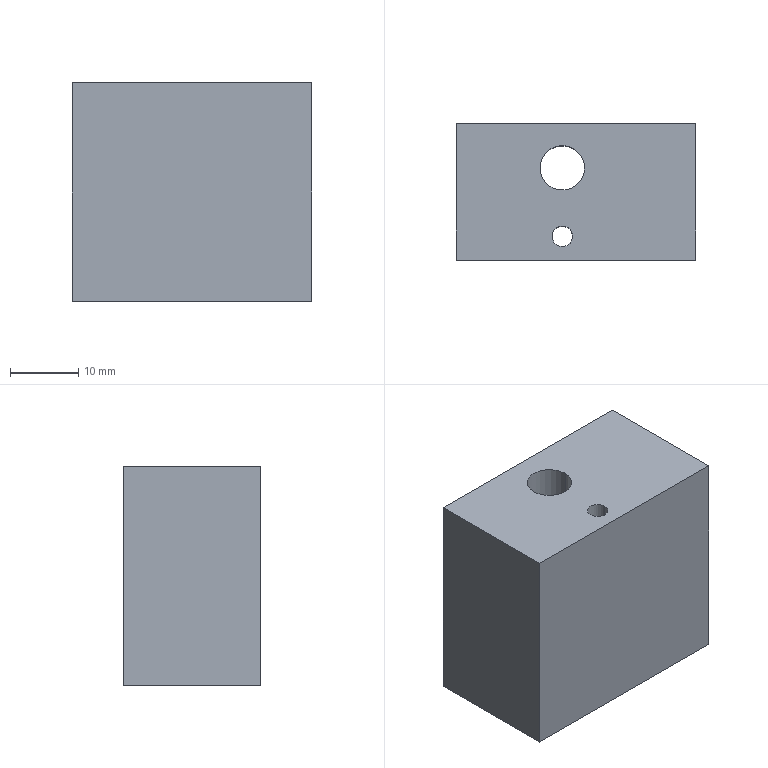Part | SolidWorks | features Cut 2, Extrusion 1, HoleWzd 1 | 1 solid | 18 faces | box 35 x 20 x 32 mm | volume 21036 mm3 | cylinder 8 | plane 6 | cone 4 | commonest cylinder face diameters 2.5 x4 3 x2 6.5 x2
STEP:
#1=CARTESIAN_POINT('',(-8.,12.5,-2.25));
#2=VERTEX_POINT('',#1);
#3=CARTESIAN_POINT('',(-8.,12.5,0.25));
#4=VERTEX_POINT('',#3);
#5=CARTESIAN_POINT('',(-8.,12.5,-1.));
#6=DIRECTION('',(0.,1.,0.));
#7=DIRECTION('',(0.,0.,1.));
#8=AXIS2_PLACEMENT_3D('',#5,#6,#7);
#9=CIRCLE('',#8,1.25);
#10=EDGE_CURVE('',#2,#4,#9,.T.);
#11=ORIENTED_EDGE('',*,*,#10,.F.);
#12=CARTESIAN_POINT('',(-8.,20.,-2.25));
#13=VERTEX_POINT('',#12);
#14=CARTESIAN_POINT('',(-8.,20.,-2.25));
#15=DIRECTION('',(0.,1.,0.));
#16=VECTOR('',#15,1000.);
#17=LINE('',#14,#16);
#18=EDGE_CURVE('',#2,#13,#17,.T.);
#19=ORIENTED_EDGE('',*,*,#18,.T.);
#20=CARTESIAN_POINT('',(-8.,20.,0.25));
#21=VERTEX_POINT('',#20);
#22=CARTESIAN_POINT('',(-8.,20.,-1.));
#23=DIRECTION('',(0.,1.,0.));
#24=DIRECTION('',(0.,0.,1.));
#25=AXIS2_PLACEMENT_3D('',#22,#23,#24);
#26=CIRCLE('',#25,1.25);
#27=EDGE_CURVE('',#13,#21,#26,.T.);
#28=ORIENTED_EDGE('',*,*,#27,.T.);
#29=CARTESIAN_POINT('',(-8.,20.,0.25));
#30=DIRECTION('',(0.,1.,0.));
#31=VECTOR('',#30,1000.);
#32=LINE('',#29,#31);
#33=EDGE_CURVE('',#4,#21,#32,.T.);
#34=ORIENTED_EDGE('',*,*,#33,.F.);
#35=EDGE_LOOP('',(#11,#19,#28,#34));
#36=FACE_OUTER_BOUND('',#35,.T.);
#37=CARTESIAN_POINT('',(-8.,20.,-1.));
#38=DIRECTION('',(0.,1.,0.));
#39=DIRECTION('',(0.,0.,1.));
#40=AXIS2_PLACEMENT_3D('',#37,#38,#39);
#41=CYLINDRICAL_SURFACE('',#40,1.25);
#42=ADVANCED_FACE('',(#36),#41,.F.);
#43=CARTESIAN_POINT('',(-8.,11.749,-1.));
#44=VERTEX_POINT('',#43);
#45=CARTESIAN_POINT('',(-8.,12.5,0.25));
#46=DIRECTION('',(0.,0.515,0.8572));
#47=VECTOR('',#46,1000.);
#48=LINE('',#45,#47);
#49=EDGE_CURVE('',#44,#4,#48,.T.);
#50=ORIENTED_EDGE('',*,*,#49,.F.);
#51=CARTESIAN_POINT('',(-8.,12.5,-2.25));
#52=DIRECTION('',(0.,0.515,-0.8572));
#53=VECTOR('',#52,1000.);
#54=LINE('',#51,#53);
#55=EDGE_CURVE('',#44,#2,#54,.T.);
#56=ORIENTED_EDGE('',*,*,#55,.T.);
#57=ORIENTED_EDGE('',*,*,#10,.T.);
#58=EDGE_LOOP('',(#50,#56,#57));
#59=FACE_OUTER_BOUND('',#58,.T.);
#60=CARTESIAN_POINT('',(-8.,12.5,-1.));
#61=DIRECTION('',(0.,1.,0.));
#62=DIRECTION('',(0.,0.,1.));
#63=AXIS2_PLACEMENT_3D('',#60,#61,#62);
#64=CONICAL_SURFACE('',#63,1.25,1.03);
#65=ADVANCED_FACE('',(#59),#64,.F.);
#66=CARTESIAN_POINT('',(-14.5,12.5,-2.25));
#67=VERTEX_POINT('',#66);
#68=CARTESIAN_POINT('',(-14.5,12.5,0.25));
#69=VERTEX_POINT('',#68);
#70=CARTESIAN_POINT('',(-14.5,12.5,-1.));
#71=DIRECTION('',(0.,1.,0.));
#72=DIRECTION('',(0.,0.,1.));
#73=AXIS2_PLACEMENT_3D('',#70,#71,#72);
#74=CIRCLE('',#73,1.25);
#75=EDGE_CURVE('',#67,#69,#74,.T.);
#76=ORIENTED_EDGE('',*,*,#75,.F.);
#77=CARTESIAN_POINT('',(-14.5,20.,-2.25));
#78=VERTEX_POINT('',#77);
#79=CARTESIAN_POINT('',(-14.5,20.,-2.25));
#80=DIRECTION('',(0.,1.,0.));
#81=VECTOR('',#80,1000.);
#82=LINE('',#79,#81);
#83=EDGE_CURVE('',#67,#78,#82,.T.);
#84=ORIENTED_EDGE('',*,*,#83,.T.);
#85=CARTESIAN_POINT('',(-14.5,20.,0.25));
#86=VERTEX_POINT('',#85);
#87=CARTESIAN_POINT('',(-14.5,20.,-1.));
#88=DIRECTION('',(0.,1.,0.));
#89=DIRECTION('',(0.,0.,1.));
#90=AXIS2_PLACEMENT_3D('',#87,#88,#89);
#91=CIRCLE('',#90,1.25);
#92=EDGE_CURVE('',#78,#86,#91,.T.);
#93=ORIENTED_EDGE('',*,*,#92,.T.);
#94=CARTESIAN_POINT('',(-14.5,20.,0.25));
#95=DIRECTION('',(0.,1.,0.));
#96=VECTOR('',#95,1000.);
#97=LINE('',#94,#96);
#98=EDGE_CURVE('',#69,#86,#97,.T.);
#99=ORIENTED_EDGE('',*,*,#98,.F.);
#100=EDGE_LOOP('',(#76,#84,#93,#99));
#101=FACE_OUTER_BOUND('',#100,.T.);
#102=CARTESIAN_POINT('',(-14.5,20.,-1.));
#103=DIRECTION('',(0.,1.,0.));
#104=DIRECTION('',(0.,0.,1.));
#105=AXIS2_PLACEMENT_3D('',#102,#103,#104);
#106=CYLINDRICAL_SURFACE('',#105,1.25);
#107=ADVANCED_FACE('',(#101),#106,.F.);
#108=CARTESIAN_POINT('',(-14.5,11.749,-1.));
#109=VERTEX_POINT('',#108);
#110=CARTESIAN_POINT('',(-14.5,12.5,0.25));
#111=DIRECTION('',(0.,0.515,0.8572));
#112=VECTOR('',#111,1000.);
#113=LINE('',#110,#112);
#114=EDGE_CURVE('',#109,#69,#113,.T.);
#115=ORIENTED_EDGE('',*,*,#114,.F.);
#116=CARTESIAN_POINT('',(-14.5,12.5,-2.25));
#117=DIRECTION('',(0.,0.515,-0.8572));
#118=VECTOR('',#117,1000.);
#119=LINE('',#116,#118);
#120=EDGE_CURVE('',#109,#67,#119,.T.);
#121=ORIENTED_EDGE('',*,*,#120,.T.);
#122=ORIENTED_EDGE('',*,*,#75,.T.);
#123=EDGE_LOOP('',(#115,#121,#122));
#124=FACE_OUTER_BOUND('',#123,.T.);
#125=CARTESIAN_POINT('',(-14.5,12.5,-1.));
#126=DIRECTION('',(0.,1.,0.));
#127=DIRECTION('',(0.,0.,1.));
#128=AXIS2_PLACEMENT_3D('',#125,#126,#127);
#129=CONICAL_SURFACE('',#128,1.25,1.03);
#130=ADVANCED_FACE('',(#124),#129,.F.);
#131=CARTESIAN_POINT('',(1.25,13.5,-16.));
#132=VERTEX_POINT('',#131);
#133=CARTESIAN_POINT('',(-5.25,13.5,-16.));
#134=VERTEX_POINT('',#133);
#135=CARTESIAN_POINT('',(-2.,13.5,-16.));
#136=DIRECTION('',(0.,0.,-1.));
#137=DIRECTION('',(1.,0.,0.));
#138=AXIS2_PLACEMENT_3D('',#135,#136,#137);
#139=CIRCLE('',#138,3.25);
#140=EDGE_CURVE('',#132,#134,#139,.T.);
#141=ORIENTED_EDGE('',*,*,#140,.T.);
#142=CARTESIAN_POINT('',(-5.25,13.5,16.));
#143=VERTEX_POINT('',#142);
#144=CARTESIAN_POINT('',(-5.25,13.5,-16.001));
#145=DIRECTION('',(0.,0.,1.));
#146=VECTOR('',#145,1000.);
#147=LINE('',#144,#146);
#148=EDGE_CURVE('',#134,#143,#147,.T.);
#149=ORIENTED_EDGE('',*,*,#148,.T.);
#150=CARTESIAN_POINT('',(1.25,13.5,16.));
#151=VERTEX_POINT('',#150);
#152=CARTESIAN_POINT('',(-2.,13.5,16.));
#153=DIRECTION('',(0.,0.,1.));
#154=DIRECTION('',(1.,0.,0.));
#155=AXIS2_PLACEMENT_3D('',#152,#153,#154);
#156=CIRCLE('',#155,3.25);
#157=EDGE_CURVE('',#143,#151,#156,.T.);
#158=ORIENTED_EDGE('',*,*,#157,.T.);
#159=CARTESIAN_POINT('',(1.25,13.5,-16.001));
#160=DIRECTION('',(0.,0.,1.));
#161=VECTOR('',#160,1000.);
#162=LINE('',#159,#161);
#163=EDGE_CURVE('',#132,#151,#162,.T.);
#164=ORIENTED_EDGE('',*,*,#163,.F.);
#165=EDGE_LOOP('',(#141,#149,#158,#164));
#166=FACE_OUTER_BOUND('',#165,.T.);
#167=CARTESIAN_POINT('',(-2.,13.5,-16.001));
#168=DIRECTION('',(0.,0.,1.));
#169=DIRECTION('',(1.,0.,0.));
#170=AXIS2_PLACEMENT_3D('',#167,#168,#169);
#171=CYLINDRICAL_SURFACE('',#170,3.25);
#172=ADVANCED_FACE('',(#166),#171,.F.);
#173=CARTESIAN_POINT('',(-0.5,3.5,-16.));
#174=VERTEX_POINT('',#173);
#175=CARTESIAN_POINT('',(-3.5,3.5,-16.));
#176=VERTEX_POINT('',#175);
#177=CARTESIAN_POINT('',(-2.,3.5,-16.));
#178=DIRECTION('',(0.,0.,-1.));
#179=DIRECTION('',(1.,0.,0.));
#180=AXIS2_PLACEMENT_3D('',#177,#178,#179);
#181=CIRCLE('',#180,1.5);
#182=EDGE_CURVE('',#174,#176,#181,.T.);
#183=ORIENTED_EDGE('',*,*,#182,.T.);
#184=CARTESIAN_POINT('',(-3.5,3.5,16.));
#185=VERTEX_POINT('',#184);
#186=CARTESIAN_POINT('',(-3.5,3.5,-16.001));
#187=DIRECTION('',(0.,0.,1.));
#188=VECTOR('',#187,1000.);
#189=LINE('',#186,#188);
#190=EDGE_CURVE('',#176,#185,#189,.T.);
#191=ORIENTED_EDGE('',*,*,#190,.T.);
#192=CARTESIAN_POINT('',(-0.5,3.5,16.));
#193=VERTEX_POINT('',#192);
#194=CARTESIAN_POINT('',(-2.,3.5,16.));
#195=DIRECTION('',(0.,0.,1.));
#196=DIRECTION('',(1.,0.,0.));
#197=AXIS2_PLACEMENT_3D('',#194,#195,#196);
#198=CIRCLE('',#197,1.5);
#199=EDGE_CURVE('',#185,#193,#198,.T.);
#200=ORIENTED_EDGE('',*,*,#199,.T.);
#201=CARTESIAN_POINT('',(-0.5,3.5,-16.001));
#202=DIRECTION('',(0.,0.,1.));
#203=VECTOR('',#202,1000.);
#204=LINE('',#201,#203);
#205=EDGE_CURVE('',#174,#193,#204,.T.);
#206=ORIENTED_EDGE('',*,*,#205,.F.);
#207=EDGE_LOOP('',(#183,#191,#200,#206));
#208=FACE_OUTER_BOUND('',#207,.T.);
#209=CARTESIAN_POINT('',(-2.,3.5,-16.001));
#210=DIRECTION('',(0.,0.,1.));
#211=DIRECTION('',(1.,0.,0.));
#212=AXIS2_PLACEMENT_3D('',#209,#210,#211);
#213=CYLINDRICAL_SURFACE('',#212,1.5);
#214=ADVANCED_FACE('',(#208),#213,.F.);
#215=CARTESIAN_POINT('',(17.5,0.,16.));
#216=VERTEX_POINT('',#215);
#217=CARTESIAN_POINT('',(17.5,0.,-16.));
#218=VERTEX_POINT('',#217);
#219=CARTESIAN_POINT('',(17.5,0.,-16.));
#220=DIRECTION('',(0.,0.,-1.));
#221=VECTOR('',#220,1000.);
#222=LINE('',#219,#221);
#223=EDGE_CURVE('',#216,#218,#222,.T.);
#224=ORIENTED_EDGE('',*,*,#223,.T.);
#225=CARTESIAN_POINT('',(17.5,20.,-16.));
#226=VERTEX_POINT('',#225);
#227=CARTESIAN_POINT('',(17.5,20.,-16.));
#228=DIRECTION('',(0.,-1.,0.));
#229=VECTOR('',#228,1000.);
#230=LINE('',#227,#229);
#231=EDGE_CURVE('',#226,#218,#230,.T.);
#232=ORIENTED_EDGE('',*,*,#231,.F.);
#233=CARTESIAN_POINT('',(17.5,20.,16.));
#234=VERTEX_POINT('',#233);
#235=CARTESIAN_POINT('',(17.5,20.,-16.));
#236=DIRECTION('',(0.,0.,-1.));
#237=VECTOR('',#236,1000.);
#238=LINE('',#235,#237);
#239=EDGE_CURVE('',#234,#226,#238,.T.);
#240=ORIENTED_EDGE('',*,*,#239,.F.);
#241=CARTESIAN_POINT('',(17.5,20.,16.));
#242=DIRECTION('',(0.,-1.,0.));
#243=VECTOR('',#242,1000.);
#244=LINE('',#241,#243);
#245=EDGE_CURVE('',#234,#216,#244,.T.);
#246=ORIENTED_EDGE('',*,*,#245,.T.);
#247=EDGE_LOOP('',(#224,#232,#240,#246));
#248=FACE_OUTER_BOUND('',#247,.T.);
#249=CARTESIAN_POINT('',(17.5,20.,-16.));
#250=DIRECTION('',(-1.,0.,0.));
#251=DIRECTION('',(0.,0.,1.));
#252=AXIS2_PLACEMENT_3D('',#249,#250,#251);
#253=PLANE('',#252);
#254=ADVANCED_FACE('',(#248),#253,.F.);
#255=ORIENTED_EDGE('',*,*,#140,.F.);
#256=CARTESIAN_POINT('',(-2.,13.5,-16.));
#257=DIRECTION('',(0.,0.,-1.));
#258=DIRECTION('',(1.,0.,0.));
#259=AXIS2_PLACEMENT_3D('',#256,#257,#258);
#260=CIRCLE('',#259,3.25);
#261=EDGE_CURVE('',#134,#132,#260,.T.);
#262=ORIENTED_EDGE('',*,*,#261,.F.);
#263=EDGE_LOOP('',(#255,#262));
#264=FACE_BOUND('',#263,.T.);
#265=ORIENTED_EDGE('',*,*,#182,.F.);
#266=CARTESIAN_POINT('',(-2.,3.5,-16.));
#267=DIRECTION('',(0.,0.,-1.));
#268=DIRECTION('',(1.,0.,0.));
#269=AXIS2_PLACEMENT_3D('',#266,#267,#268);
#270=CIRCLE('',#269,1.5);
#271=EDGE_CURVE('',#176,#174,#270,.T.);
#272=ORIENTED_EDGE('',*,*,#271,.F.);
#273=EDGE_LOOP('',(#265,#272));
#274=FACE_BOUND('',#273,.T.);
#275=CARTESIAN_POINT('',(-17.5,0.,-16.));
#276=VERTEX_POINT('',#275);
#277=CARTESIAN_POINT('',(-17.5,0.,-16.));
#278=DIRECTION('',(-1.,0.,0.));
#279=VECTOR('',#278,1000.);
#280=LINE('',#277,#279);
#281=EDGE_CURVE('',#218,#276,#280,.T.);
#282=ORIENTED_EDGE('',*,*,#281,.T.);
#283=CARTESIAN_POINT('',(-17.5,20.,-16.));
#284=VERTEX_POINT('',#283);
#285=CARTESIAN_POINT('',(-17.5,20.,-16.));
#286=DIRECTION('',(0.,-1.,0.));
#287=VECTOR('',#286,1000.);
#288=LINE('',#285,#287);
#289=EDGE_CURVE('',#284,#276,#288,.T.);
#290=ORIENTED_EDGE('',*,*,#289,.F.);
#291=CARTESIAN_POINT('',(-17.5,20.,-16.));
#292=DIRECTION('',(-1.,0.,0.));
#293=VECTOR('',#292,1000.);
#294=LINE('',#291,#293);
#295=EDGE_CURVE('',#226,#284,#294,.T.);
#296=ORIENTED_EDGE('',*,*,#295,.F.);
#297=ORIENTED_EDGE('',*,*,#231,.T.);
#298=EDGE_LOOP('',(#282,#290,#296,#297));
#299=FACE_OUTER_BOUND('',#298,.T.);
#300=CARTESIAN_POINT('',(-17.5,20.,-16.));
#301=DIRECTION('',(0.,0.,1.));
#302=DIRECTION('',(1.,0.,0.));
#303=AXIS2_PLACEMENT_3D('',#300,#301,#302);
#304=PLANE('',#303);
#305=ADVANCED_FACE('',(#264,#274,#299),#304,.F.);
#306=CARTESIAN_POINT('',(-17.5,0.,16.));
#307=VERTEX_POINT('',#306);
#308=CARTESIAN_POINT('',(-17.5,0.,-16.));
#309=DIRECTION('',(0.,0.,1.));
#310=VECTOR('',#309,1000.);
#311=LINE('',#308,#310);
#312=EDGE_CURVE('',#276,#307,#311,.T.);
#313=ORIENTED_EDGE('',*,*,#312,.T.);
#314=CARTESIAN_POINT('',(-17.5,20.,16.));
#315=VERTEX_POINT('',#314);
#316=CARTESIAN_POINT('',(-17.5,20.,16.));
#317=DIRECTION('',(0.,-1.,0.));
#318=VECTOR('',#317,1000.);
#319=LINE('',#316,#318);
#320=EDGE_CURVE('',#315,#307,#319,.T.);
#321=ORIENTED_EDGE('',*,*,#320,.F.);
#322=CARTESIAN_POINT('',(-17.5,20.,-16.));
#323=DIRECTION('',(0.,0.,1.));
#324=VECTOR('',#323,1000.);
#325=LINE('',#322,#324);
#326=EDGE_CURVE('',#284,#315,#325,.T.);
#327=ORIENTED_EDGE('',*,*,#326,.F.);
#328=ORIENTED_EDGE('',*,*,#289,.T.);
#329=EDGE_LOOP('',(#313,#321,#327,#328));
#330=FACE_OUTER_BOUND('',#329,.T.);
#331=CARTESIAN_POINT('',(-17.5,20.,-16.));
#332=DIRECTION('',(1.,0.,0.));
#333=DIRECTION('',(0.,0.,-1.));
#334=AXIS2_PLACEMENT_3D('',#331,#332,#333);
#335=PLANE('',#334);
#336=ADVANCED_FACE('',(#330),#335,.F.);
#337=CARTESIAN_POINT('',(-2.,13.5,16.));
#338=DIRECTION('',(0.,0.,1.));
#339=DIRECTION('',(1.,0.,0.));
#340=AXIS2_PLACEMENT_3D('',#337,#338,#339);
#341=CIRCLE('',#340,3.25);
#342=EDGE_CURVE('',#151,#143,#341,.T.);
#343=ORIENTED_EDGE('',*,*,#342,.F.);
#344=ORIENTED_EDGE('',*,*,#157,.F.);
#345=EDGE_LOOP('',(#343,#344));
#346=FACE_BOUND('',#345,.T.);
#347=CARTESIAN_POINT('',(-2.,3.5,16.));
#348=DIRECTION('',(0.,0.,1.));
#349=DIRECTION('',(1.,0.,0.));
#350=AXIS2_PLACEMENT_3D('',#347,#348,#349);
#351=CIRCLE('',#350,1.5);
#352=EDGE_CURVE('',#193,#185,#351,.T.);
#353=ORIENTED_EDGE('',*,*,#352,.F.);
#354=ORIENTED_EDGE('',*,*,#199,.F.);
#355=EDGE_LOOP('',(#353,#354));
#356=FACE_BOUND('',#355,.T.);
#357=CARTESIAN_POINT('',(-17.5,0.,16.));
#358=DIRECTION('',(1.,0.,0.));
#359=VECTOR('',#358,1000.);
#360=LINE('',#357,#359);
#361=EDGE_CURVE('',#307,#216,#360,.T.);
#362=ORIENTED_EDGE('',*,*,#361,.T.);
#363=ORIENTED_EDGE('',*,*,#245,.F.);
#364=CARTESIAN_POINT('',(-17.5,20.,16.));
#365=DIRECTION('',(1.,0.,0.));
#366=VECTOR('',#365,1000.);
#367=LINE('',#364,#366);
#368=EDGE_CURVE('',#315,#234,#367,.T.);
#369=ORIENTED_EDGE('',*,*,#368,.F.);
#370=ORIENTED_EDGE('',*,*,#320,.T.);
#371=EDGE_LOOP('',(#362,#363,#369,#370));
#372=FACE_OUTER_BOUND('',#371,.T.);
#373=CARTESIAN_POINT('',(-17.5,20.,16.));
#374=DIRECTION('',(0.,0.,-1.));
#375=DIRECTION('',(-1.,0.,0.));
#376=AXIS2_PLACEMENT_3D('',#373,#374,#375);
#377=PLANE('',#376);
#378=ADVANCED_FACE('',(#346,#356,#372),#377,.F.);
#379=CARTESIAN_POINT('',(-8.,20.,-1.));
#380=DIRECTION('',(0.,1.,0.));
#381=DIRECTION('',(0.,0.,1.));
#382=AXIS2_PLACEMENT_3D('',#379,#380,#381);
#383=CIRCLE('',#382,1.25);
#384=EDGE_CURVE('',#21,#13,#383,.T.);
#385=ORIENTED_EDGE('',*,*,#384,.F.);
#386=ORIENTED_EDGE('',*,*,#27,.F.);
#387=EDGE_LOOP('',(#385,#386));
#388=FACE_BOUND('',#387,.T.);
#389=CARTESIAN_POINT('',(-14.5,20.,-1.));
#390=DIRECTION('',(0.,1.,0.));
#391=DIRECTION('',(0.,0.,1.));
#392=AXIS2_PLACEMENT_3D('',#389,#390,#391);
#393=CIRCLE('',#392,1.25);
#394=EDGE_CURVE('',#86,#78,#393,.T.);
#395=ORIENTED_EDGE('',*,*,#394,.F.);
#396=ORIENTED_EDGE('',*,*,#92,.F.);
#397=EDGE_LOOP('',(#395,#396));
#398=FACE_BOUND('',#397,.T.);
#399=ORIENTED_EDGE('',*,*,#239,.T.);
#400=ORIENTED_EDGE('',*,*,#295,.T.);
#401=ORIENTED_EDGE('',*,*,#326,.T.);
#402=ORIENTED_EDGE('',*,*,#368,.T.);
#403=EDGE_LOOP('',(#399,#400,#401,#402));
#404=FACE_OUTER_BOUND('',#403,.T.);
#405=CARTESIAN_POINT('',(0.,20.,0.));
#406=DIRECTION('',(0.,1.,0.));
#407=DIRECTION('',(0.,0.,1.));
#408=AXIS2_PLACEMENT_3D('',#405,#406,#407);
#409=PLANE('',#408);
#410=ADVANCED_FACE('',(#388,#398,#404),#409,.T.);
#411=ORIENTED_EDGE('',*,*,#223,.F.);
#412=ORIENTED_EDGE('',*,*,#361,.F.);
#413=ORIENTED_EDGE('',*,*,#312,.F.);
#414=ORIENTED_EDGE('',*,*,#281,.F.);
#415=EDGE_LOOP('',(#411,#412,#413,#414));
#416=FACE_OUTER_BOUND('',#415,.T.);
#417=CARTESIAN_POINT('',(0.,0.,0.));
#418=DIRECTION('',(0.,1.,0.));
#419=DIRECTION('',(0.,0.,1.));
#420=AXIS2_PLACEMENT_3D('',#417,#418,#419);
#421=PLANE('',#420);
#422=ADVANCED_FACE('',(#416),#421,.F.);
#423=ORIENTED_EDGE('',*,*,#190,.F.);
#424=ORIENTED_EDGE('',*,*,#271,.T.);
#425=ORIENTED_EDGE('',*,*,#205,.T.);
#426=ORIENTED_EDGE('',*,*,#352,.T.);
#427=EDGE_LOOP('',(#423,#424,#425,#426));
#428=FACE_OUTER_BOUND('',#427,.T.);
#429=CARTESIAN_POINT('',(-2.,3.5,-16.001));
#430=DIRECTION('',(0.,0.,1.));
#431=DIRECTION('',(1.,0.,0.));
#432=AXIS2_PLACEMENT_3D('',#429,#430,#431);
#433=CYLINDRICAL_SURFACE('',#432,1.5);
#434=ADVANCED_FACE('',(#428),#433,.F.);
#435=ORIENTED_EDGE('',*,*,#148,.F.);
#436=ORIENTED_EDGE('',*,*,#261,.T.);
#437=ORIENTED_EDGE('',*,*,#163,.T.);
#438=ORIENTED_EDGE('',*,*,#342,.T.);
#439=EDGE_LOOP('',(#435,#436,#437,#438));
#440=FACE_OUTER_BOUND('',#439,.T.);
#441=CARTESIAN_POINT('',(-2.,13.5,-16.001));
#442=DIRECTION('',(0.,0.,1.));
#443=DIRECTION('',(1.,0.,0.));
#444=AXIS2_PLACEMENT_3D('',#441,#442,#443);
#445=CYLINDRICAL_SURFACE('',#444,3.25);
#446=ADVANCED_FACE('',(#440),#445,.F.);
#447=ORIENTED_EDGE('',*,*,#120,.F.);
#448=ORIENTED_EDGE('',*,*,#114,.T.);
#449=CARTESIAN_POINT('',(-14.5,12.5,-1.));
#450=DIRECTION('',(0.,1.,0.));
#451=DIRECTION('',(0.,0.,1.));
#452=AXIS2_PLACEMENT_3D('',#449,#450,#451);
#453=CIRCLE('',#452,1.25);
#454=EDGE_CURVE('',#69,#67,#453,.T.);
#455=ORIENTED_EDGE('',*,*,#454,.T.);
#456=EDGE_LOOP('',(#447,#448,#455));
#457=FACE_OUTER_BOUND('',#456,.T.);
#458=CARTESIAN_POINT('',(-14.5,12.5,-1.));
#459=DIRECTION('',(0.,1.,0.));
#460=DIRECTION('',(0.,0.,1.));
#461=AXIS2_PLACEMENT_3D('',#458,#459,#460);
#462=CONICAL_SURFACE('',#461,1.25,1.03);
#463=ADVANCED_FACE('',(#457),#462,.F.);
#464=ORIENTED_EDGE('',*,*,#83,.F.);
#465=ORIENTED_EDGE('',*,*,#454,.F.);
#466=ORIENTED_EDGE('',*,*,#98,.T.);
#467=ORIENTED_EDGE('',*,*,#394,.T.);
#468=EDGE_LOOP('',(#464,#465,#466,#467));
#469=FACE_OUTER_BOUND('',#468,.T.);
#470=CARTESIAN_POINT('',(-14.5,20.,-1.));
#471=DIRECTION('',(0.,1.,0.));
#472=DIRECTION('',(0.,0.,1.));
#473=AXIS2_PLACEMENT_3D('',#470,#471,#472);
#474=CYLINDRICAL_SURFACE('',#473,1.25);
#475=ADVANCED_FACE('',(#469),#474,.F.);
#476=ORIENTED_EDGE('',*,*,#55,.F.);
#477=ORIENTED_EDGE('',*,*,#49,.T.);
#478=CARTESIAN_POINT('',(-8.,12.5,-1.));
#479=DIRECTION('',(0.,1.,0.));
#480=DIRECTION('',(0.,0.,1.));
#481=AXIS2_PLACEMENT_3D('',#478,#479,#480);
#482=CIRCLE('',#481,1.25);
#483=EDGE_CURVE('',#4,#2,#482,.T.);
#484=ORIENTED_EDGE('',*,*,#483,.T.);
#485=EDGE_LOOP('',(#476,#477,#484));
#486=FACE_OUTER_BOUND('',#485,.T.);
#487=CARTESIAN_POINT('',(-8.,12.5,-1.));
#488=DIRECTION('',(0.,1.,0.));
#489=DIRECTION('',(0.,0.,1.));
#490=AXIS2_PLACEMENT_3D('',#487,#488,#489);
#491=CONICAL_SURFACE('',#490,1.25,1.03);
#492=ADVANCED_FACE('',(#486),#491,.F.);
#493=ORIENTED_EDGE('',*,*,#18,.F.);
#494=ORIENTED_EDGE('',*,*,#483,.F.);
#495=ORIENTED_EDGE('',*,*,#33,.T.);
#496=ORIENTED_EDGE('',*,*,#384,.T.);
#497=EDGE_LOOP('',(#493,#494,#495,#496));
#498=FACE_OUTER_BOUND('',#497,.T.);
#499=CARTESIAN_POINT('',(-8.,20.,-1.));
#500=DIRECTION('',(0.,1.,0.));
#501=DIRECTION('',(0.,0.,1.));
#502=AXIS2_PLACEMENT_3D('',#499,#500,#501);
#503=CYLINDRICAL_SURFACE('',#502,1.25);
#504=ADVANCED_FACE('',(#498),#503,.F.);
#505=CLOSED_SHELL('',(#42,#65,#107,#130,#172,#214,#254,#305,#336,#378,#410,#422,#434,#446,#463,#475,#492,#504));
#506=MANIFOLD_SOLID_BREP('',#505);
#507=CARTESIAN_POINT('',(0.,0.,0.));
#508=DIRECTION('',(0.,0.,1.));
#509=DIRECTION('',(1.,0.,0.));
#510=AXIS2_PLACEMENT_3D('',#507,#508,#509);
#511=(LENGTH_UNIT()NAMED_UNIT(*)SI_UNIT(.MILLI.,.METRE.));
#512=UNCERTAINTY_MEASURE_WITH_UNIT(LENGTH_MEASURE(0.00001),#511,'','');
#513=(NAMED_UNIT(*)PLANE_ANGLE_UNIT()SI_UNIT($,.RADIAN.));
#514=(NAMED_UNIT(*)SI_UNIT($,.STERADIAN.)SOLID_ANGLE_UNIT());
#515=(GEOMETRIC_REPRESENTATION_CONTEXT(3)GLOBAL_UNCERTAINTY_ASSIGNED_CONTEXT((#512))GLOBAL_UNIT_ASSIGNED_CONTEXT((#511,#513,#514))REPRESENTATION_CONTEXT('',''));
#516=ADVANCED_BREP_SHAPE_REPRESENTATION('',(#506,#510),#515);